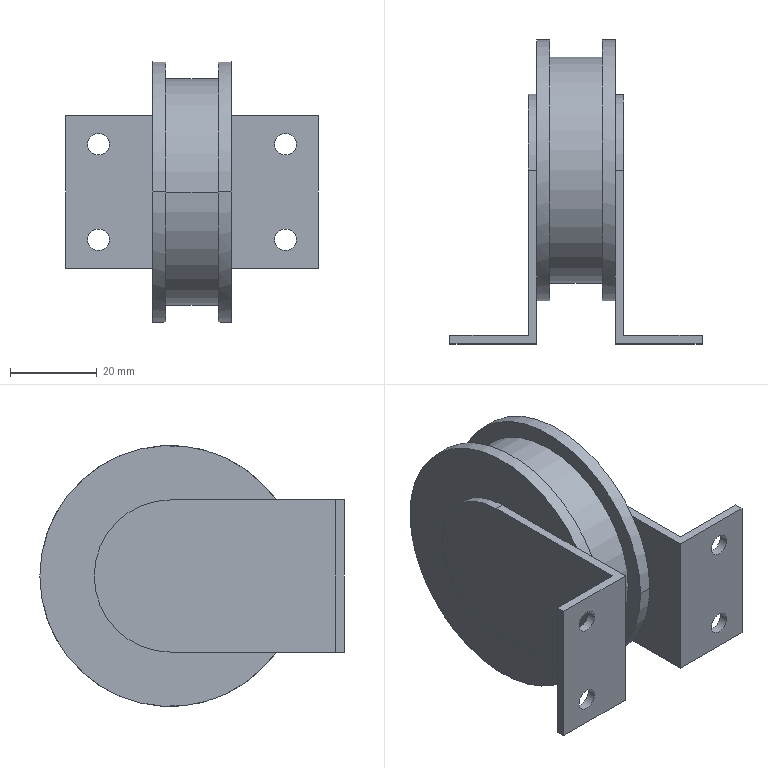Part | SolidWorks | features ICE 3, MirrorPattern 1, Revolution 1 | 1 solid | 35 faces | box 58 x 70 x 60 mm | volume 52336 mm3 | plane 18 | cylinder 17 | commonest cylinder face diameters 5 x8 60 x4 35 x3 52 x2
STEP:
#1=CARTESIAN_POINT('',(33.,-38.,11.));
#2=VERTEX_POINT('',#1);
#3=CARTESIAN_POINT('',(28.,-38.,11.));
#4=VERTEX_POINT('',#3);
#5=CARTESIAN_POINT('',(30.5,-38.,11.));
#6=DIRECTION('',(0.,1.,0.));
#7=DIRECTION('',(1.,0.,0.));
#8=AXIS2_PLACEMENT_3D('',#5,#6,#7);
#9=CIRCLE('',#8,2.5);
#10=EDGE_CURVE('',#2,#4,#9,.T.);
#11=ORIENTED_EDGE('',*,*,#10,.T.);
#12=CARTESIAN_POINT('',(28.,-40.,11.));
#13=VERTEX_POINT('',#12);
#14=CARTESIAN_POINT('',(28.,30.001,11.));
#15=DIRECTION('',(0.,-1.,0.));
#16=VECTOR('',#15,1000.);
#17=LINE('',#14,#16);
#18=EDGE_CURVE('',#4,#13,#17,.T.);
#19=ORIENTED_EDGE('',*,*,#18,.T.);
#20=CARTESIAN_POINT('',(33.,-40.,11.));
#21=VERTEX_POINT('',#20);
#22=CARTESIAN_POINT('',(30.5,-40.,11.));
#23=DIRECTION('',(0.,-1.,0.));
#24=DIRECTION('',(-1.,0.,0.));
#25=AXIS2_PLACEMENT_3D('',#22,#23,#24);
#26=CIRCLE('',#25,2.5);
#27=EDGE_CURVE('',#13,#21,#26,.T.);
#28=ORIENTED_EDGE('',*,*,#27,.T.);
#29=CARTESIAN_POINT('',(33.,30.001,11.));
#30=DIRECTION('',(0.,-1.,0.));
#31=VECTOR('',#30,1000.);
#32=LINE('',#29,#31);
#33=EDGE_CURVE('',#2,#21,#32,.T.);
#34=ORIENTED_EDGE('',*,*,#33,.F.);
#35=EDGE_LOOP('',(#11,#19,#28,#34));
#36=FACE_OUTER_BOUND('',#35,.T.);
#37=CARTESIAN_POINT('',(30.5,30.001,11.));
#38=DIRECTION('',(0.,-1.,0.));
#39=DIRECTION('',(1.,0.,0.));
#40=AXIS2_PLACEMENT_3D('',#37,#38,#39);
#41=CYLINDRICAL_SURFACE('',#40,2.5);
#42=ADVANCED_FACE('',(#36),#41,.F.);
#43=CARTESIAN_POINT('',(33.,-38.,-11.));
#44=VERTEX_POINT('',#43);
#45=CARTESIAN_POINT('',(28.,-38.,-11.));
#46=VERTEX_POINT('',#45);
#47=CARTESIAN_POINT('',(30.5,-38.,-11.));
#48=DIRECTION('',(0.,1.,0.));
#49=DIRECTION('',(1.,0.,0.));
#50=AXIS2_PLACEMENT_3D('',#47,#48,#49);
#51=CIRCLE('',#50,2.5);
#52=EDGE_CURVE('',#44,#46,#51,.T.);
#53=ORIENTED_EDGE('',*,*,#52,.T.);
#54=CARTESIAN_POINT('',(28.,-40.,-11.));
#55=VERTEX_POINT('',#54);
#56=CARTESIAN_POINT('',(28.,30.001,-11.));
#57=DIRECTION('',(0.,-1.,0.));
#58=VECTOR('',#57,1000.);
#59=LINE('',#56,#58);
#60=EDGE_CURVE('',#46,#55,#59,.T.);
#61=ORIENTED_EDGE('',*,*,#60,.T.);
#62=CARTESIAN_POINT('',(33.,-40.,-11.));
#63=VERTEX_POINT('',#62);
#64=CARTESIAN_POINT('',(30.5,-40.,-11.));
#65=DIRECTION('',(0.,-1.,0.));
#66=DIRECTION('',(1.,0.,0.));
#67=AXIS2_PLACEMENT_3D('',#64,#65,#66);
#68=CIRCLE('',#67,2.5);
#69=EDGE_CURVE('',#55,#63,#68,.T.);
#70=ORIENTED_EDGE('',*,*,#69,.T.);
#71=CARTESIAN_POINT('',(33.,30.001,-11.));
#72=DIRECTION('',(0.,-1.,0.));
#73=VECTOR('',#72,1000.);
#74=LINE('',#71,#73);
#75=EDGE_CURVE('',#44,#63,#74,.T.);
#76=ORIENTED_EDGE('',*,*,#75,.F.);
#77=EDGE_LOOP('',(#53,#61,#70,#76));
#78=FACE_OUTER_BOUND('',#77,.T.);
#79=CARTESIAN_POINT('',(30.5,30.001,-11.));
#80=DIRECTION('',(0.,-1.,0.));
#81=DIRECTION('',(1.,0.,0.));
#82=AXIS2_PLACEMENT_3D('',#79,#80,#81);
#83=CYLINDRICAL_SURFACE('',#82,2.5);
#84=ADVANCED_FACE('',(#78),#83,.F.);
#85=CARTESIAN_POINT('',(-15.,-38.,-11.));
#86=VERTEX_POINT('',#85);
#87=CARTESIAN_POINT('',(-10.,-38.,-11.));
#88=VERTEX_POINT('',#87);
#89=CARTESIAN_POINT('',(-12.5,-38.,-11.));
#90=DIRECTION('',(0.,-1.,0.));
#91=DIRECTION('',(-1.,0.,0.));
#92=AXIS2_PLACEMENT_3D('',#89,#90,#91);
#93=CIRCLE('',#92,2.5);
#94=EDGE_CURVE('',#86,#88,#93,.T.);
#95=ORIENTED_EDGE('',*,*,#94,.F.);
#96=CARTESIAN_POINT('',(-15.,-40.,-11.));
#97=VERTEX_POINT('',#96);
#98=CARTESIAN_POINT('',(-15.,30.001,-11.));
#99=DIRECTION('',(0.,-1.,0.));
#100=VECTOR('',#99,1000.);
#101=LINE('',#98,#100);
#102=EDGE_CURVE('',#86,#97,#101,.T.);
#103=ORIENTED_EDGE('',*,*,#102,.T.);
#104=CARTESIAN_POINT('',(-10.,-40.,-11.));
#105=VERTEX_POINT('',#104);
#106=CARTESIAN_POINT('',(-12.5,-40.,-11.));
#107=DIRECTION('',(0.,-1.,0.));
#108=DIRECTION('',(-1.,0.,0.));
#109=AXIS2_PLACEMENT_3D('',#106,#107,#108);
#110=CIRCLE('',#109,2.5);
#111=EDGE_CURVE('',#97,#105,#110,.T.);
#112=ORIENTED_EDGE('',*,*,#111,.T.);
#113=CARTESIAN_POINT('',(-10.,30.001,-11.));
#114=DIRECTION('',(0.,-1.,0.));
#115=VECTOR('',#114,1000.);
#116=LINE('',#113,#115);
#117=EDGE_CURVE('',#88,#105,#116,.T.);
#118=ORIENTED_EDGE('',*,*,#117,.F.);
#119=EDGE_LOOP('',(#95,#103,#112,#118));
#120=FACE_OUTER_BOUND('',#119,.T.);
#121=CARTESIAN_POINT('',(-12.5,30.001,-11.));
#122=DIRECTION('',(0.,-1.,0.));
#123=DIRECTION('',(1.,0.,0.));
#124=AXIS2_PLACEMENT_3D('',#121,#122,#123);
#125=CYLINDRICAL_SURFACE('',#124,2.5);
#126=ADVANCED_FACE('',(#120),#125,.F.);
#127=CARTESIAN_POINT('',(-15.,-38.,11.));
#128=VERTEX_POINT('',#127);
#129=CARTESIAN_POINT('',(-10.,-38.,11.));
#130=VERTEX_POINT('',#129);
#131=CARTESIAN_POINT('',(-12.5,-38.,11.));
#132=DIRECTION('',(0.,-1.,0.));
#133=DIRECTION('',(-1.,0.,0.));
#134=AXIS2_PLACEMENT_3D('',#131,#132,#133);
#135=CIRCLE('',#134,2.5);
#136=EDGE_CURVE('',#128,#130,#135,.T.);
#137=ORIENTED_EDGE('',*,*,#136,.F.);
#138=CARTESIAN_POINT('',(-15.,-40.,11.));
#139=VERTEX_POINT('',#138);
#140=CARTESIAN_POINT('',(-15.,30.001,11.));
#141=DIRECTION('',(0.,-1.,0.));
#142=VECTOR('',#141,1000.);
#143=LINE('',#140,#142);
#144=EDGE_CURVE('',#128,#139,#143,.T.);
#145=ORIENTED_EDGE('',*,*,#144,.T.);
#146=CARTESIAN_POINT('',(-10.,-40.,11.));
#147=VERTEX_POINT('',#146);
#148=CARTESIAN_POINT('',(-12.5,-40.,11.));
#149=DIRECTION('',(0.,-1.,0.));
#150=DIRECTION('',(1.,0.,0.));
#151=AXIS2_PLACEMENT_3D('',#148,#149,#150);
#152=CIRCLE('',#151,2.5);
#153=EDGE_CURVE('',#139,#147,#152,.T.);
#154=ORIENTED_EDGE('',*,*,#153,.T.);
#155=CARTESIAN_POINT('',(-10.,30.001,11.));
#156=DIRECTION('',(0.,-1.,0.));
#157=VECTOR('',#156,1000.);
#158=LINE('',#155,#157);
#159=EDGE_CURVE('',#130,#147,#158,.T.);
#160=ORIENTED_EDGE('',*,*,#159,.F.);
#161=EDGE_LOOP('',(#137,#145,#154,#160));
#162=FACE_OUTER_BOUND('',#161,.T.);
#163=CARTESIAN_POINT('',(-12.5,30.001,11.));
#164=DIRECTION('',(0.,-1.,0.));
#165=DIRECTION('',(1.,0.,0.));
#166=AXIS2_PLACEMENT_3D('',#163,#164,#165);
#167=CYLINDRICAL_SURFACE('',#166,2.5);
#168=ADVANCED_FACE('',(#162),#167,.F.);
#169=CARTESIAN_POINT('',(-2.,0.,-17.5));
#170=VERTEX_POINT('',#169);
#171=CARTESIAN_POINT('',(-2.,17.5,0.));
#172=VERTEX_POINT('',#171);
#173=CARTESIAN_POINT('',(-2.,0.,0.));
#174=DIRECTION('',(1.,0.,0.));
#175=DIRECTION('',(0.,1.,0.));
#176=AXIS2_PLACEMENT_3D('',#173,#174,#175);
#177=CIRCLE('',#176,17.5);
#178=EDGE_CURVE('',#170,#172,#177,.T.);
#179=ORIENTED_EDGE('',*,*,#178,.T.);
#180=CARTESIAN_POINT('',(0.,17.5,0.));
#181=VERTEX_POINT('',#180);
#182=CARTESIAN_POINT('',(-2.,17.5,0.));
#183=DIRECTION('',(1.,0.,0.));
#184=VECTOR('',#183,1000.);
#185=LINE('',#182,#184);
#186=EDGE_CURVE('',#172,#181,#185,.T.);
#187=ORIENTED_EDGE('',*,*,#186,.T.);
#188=CARTESIAN_POINT('',(0.,0.,-17.5));
#189=VERTEX_POINT('',#188);
#190=CARTESIAN_POINT('',(0.,0.,0.));
#191=DIRECTION('',(1.,0.,0.));
#192=DIRECTION('',(0.,1.,0.));
#193=AXIS2_PLACEMENT_3D('',#190,#191,#192);
#194=CIRCLE('',#193,17.5);
#195=EDGE_CURVE('',#189,#181,#194,.T.);
#196=ORIENTED_EDGE('',*,*,#195,.F.);
#197=CARTESIAN_POINT('',(-2.,0.,-17.5));
#198=DIRECTION('',(1.,0.,0.));
#199=VECTOR('',#198,1000.);
#200=LINE('',#197,#199);
#201=EDGE_CURVE('',#170,#189,#200,.T.);
#202=ORIENTED_EDGE('',*,*,#201,.F.);
#203=EDGE_LOOP('',(#179,#187,#196,#202));
#204=FACE_OUTER_BOUND('',#203,.T.);
#205=CARTESIAN_POINT('',(-2.,0.,0.));
#206=DIRECTION('',(1.,0.,0.));
#207=DIRECTION('',(0.,1.,0.));
#208=AXIS2_PLACEMENT_3D('',#205,#206,#207);
#209=CYLINDRICAL_SURFACE('',#208,17.5);
#210=ADVANCED_FACE('',(#204),#209,.T.);
#211=CARTESIAN_POINT('',(3.,26.,0.));
#212=VERTEX_POINT('',#211);
#213=CARTESIAN_POINT('',(3.,-26.,0.));
#214=VERTEX_POINT('',#213);
#215=CARTESIAN_POINT('',(3.,0.,0.));
#216=DIRECTION('',(1.,0.,0.));
#217=DIRECTION('',(0.,1.,0.));
#218=AXIS2_PLACEMENT_3D('',#215,#216,#217);
#219=CIRCLE('',#218,26.);
#220=EDGE_CURVE('',#212,#214,#219,.T.);
#221=ORIENTED_EDGE('',*,*,#220,.T.);
#222=CARTESIAN_POINT('',(15.,-26.,0.));
#223=VERTEX_POINT('',#222);
#224=CARTESIAN_POINT('',(18.,-26.,0.));
#225=DIRECTION('',(1.,0.,0.));
#226=VECTOR('',#225,1000.);
#227=LINE('',#224,#226);
#228=EDGE_CURVE('',#214,#223,#227,.T.);
#229=ORIENTED_EDGE('',*,*,#228,.T.);
#230=CARTESIAN_POINT('',(15.,26.,0.));
#231=VERTEX_POINT('',#230);
#232=CARTESIAN_POINT('',(15.,0.,0.));
#233=DIRECTION('',(1.,0.,0.));
#234=DIRECTION('',(0.,1.,0.));
#235=AXIS2_PLACEMENT_3D('',#232,#233,#234);
#236=CIRCLE('',#235,26.);
#237=EDGE_CURVE('',#231,#223,#236,.T.);
#238=ORIENTED_EDGE('',*,*,#237,.F.);
#239=CARTESIAN_POINT('',(18.,26.,0.));
#240=DIRECTION('',(1.,0.,0.));
#241=VECTOR('',#240,1000.);
#242=LINE('',#239,#241);
#243=EDGE_CURVE('',#212,#231,#242,.T.);
#244=ORIENTED_EDGE('',*,*,#243,.F.);
#245=EDGE_LOOP('',(#221,#229,#238,#244));
#246=FACE_OUTER_BOUND('',#245,.T.);
#247=CARTESIAN_POINT('',(18.,0.,0.));
#248=DIRECTION('',(1.,0.,0.));
#249=DIRECTION('',(0.,1.,0.));
#250=AXIS2_PLACEMENT_3D('',#247,#248,#249);
#251=CYLINDRICAL_SURFACE('',#250,26.);
#252=ADVANCED_FACE('',(#246),#251,.T.);
#253=CARTESIAN_POINT('',(15.,30.,0.));
#254=VERTEX_POINT('',#253);
#255=CARTESIAN_POINT('',(15.,-30.,0.));
#256=VERTEX_POINT('',#255);
#257=CARTESIAN_POINT('',(15.,0.,0.));
#258=DIRECTION('',(1.,0.,0.));
#259=DIRECTION('',(0.,1.,0.));
#260=AXIS2_PLACEMENT_3D('',#257,#258,#259);
#261=CIRCLE('',#260,30.);
#262=EDGE_CURVE('',#254,#256,#261,.T.);
#263=ORIENTED_EDGE('',*,*,#262,.T.);
#264=CARTESIAN_POINT('',(18.,-30.,0.));
#265=VERTEX_POINT('',#264);
#266=CARTESIAN_POINT('',(18.,-30.,0.));
#267=DIRECTION('',(1.,0.,0.));
#268=VECTOR('',#267,1000.);
#269=LINE('',#266,#268);
#270=EDGE_CURVE('',#256,#265,#269,.T.);
#271=ORIENTED_EDGE('',*,*,#270,.T.);
#272=CARTESIAN_POINT('',(18.,-24.367,17.5));
#273=VERTEX_POINT('',#272);
#274=CARTESIAN_POINT('',(18.,0.,0.));
#275=DIRECTION('',(1.,0.,0.));
#276=DIRECTION('',(0.,1.,0.));
#277=AXIS2_PLACEMENT_3D('',#274,#275,#276);
#278=CIRCLE('',#277,30.);
#279=EDGE_CURVE('',#273,#265,#278,.T.);
#280=ORIENTED_EDGE('',*,*,#279,.F.);
#281=CARTESIAN_POINT('',(18.,30.,0.));
#282=VERTEX_POINT('',#281);
#283=CARTESIAN_POINT('',(18.,0.,0.));
#284=DIRECTION('',(1.,0.,0.));
#285=DIRECTION('',(0.,1.,0.));
#286=AXIS2_PLACEMENT_3D('',#283,#284,#285);
#287=CIRCLE('',#286,30.);
#288=EDGE_CURVE('',#282,#273,#287,.T.);
#289=ORIENTED_EDGE('',*,*,#288,.F.);
#290=CARTESIAN_POINT('',(18.,30.,0.));
#291=DIRECTION('',(1.,0.,0.));
#292=VECTOR('',#291,1000.);
#293=LINE('',#290,#292);
#294=EDGE_CURVE('',#254,#282,#293,.T.);
#295=ORIENTED_EDGE('',*,*,#294,.F.);
#296=EDGE_LOOP('',(#263,#271,#280,#289,#295));
#297=FACE_OUTER_BOUND('',#296,.T.);
#298=CARTESIAN_POINT('',(18.,0.,0.));
#299=DIRECTION('',(1.,0.,0.));
#300=DIRECTION('',(0.,1.,0.));
#301=AXIS2_PLACEMENT_3D('',#298,#299,#300);
#302=CYLINDRICAL_SURFACE('',#301,30.);
#303=ADVANCED_FACE('',(#297),#302,.T.);
#304=CARTESIAN_POINT('',(0.,-24.367,17.5));
#305=VERTEX_POINT('',#304);
#306=CARTESIAN_POINT('',(0.,-30.,0.));
#307=VERTEX_POINT('',#306);
#308=CARTESIAN_POINT('',(0.,0.,0.));
#309=DIRECTION('',(1.,0.,0.));
#310=DIRECTION('',(0.,1.,0.));
#311=AXIS2_PLACEMENT_3D('',#308,#309,#310);
#312=CIRCLE('',#311,30.);
#313=EDGE_CURVE('',#305,#307,#312,.T.);
#314=ORIENTED_EDGE('',*,*,#313,.T.);
#315=CARTESIAN_POINT('',(3.,-30.,0.));
#316=VERTEX_POINT('',#315);
#317=CARTESIAN_POINT('',(18.,-30.,0.));
#318=DIRECTION('',(1.,0.,0.));
#319=VECTOR('',#318,1000.);
#320=LINE('',#317,#319);
#321=EDGE_CURVE('',#307,#316,#320,.T.);
#322=ORIENTED_EDGE('',*,*,#321,.T.);
#323=CARTESIAN_POINT('',(3.,30.,0.));
#324=VERTEX_POINT('',#323);
#325=CARTESIAN_POINT('',(3.,0.,0.));
#326=DIRECTION('',(1.,0.,0.));
#327=DIRECTION('',(0.,1.,0.));
#328=AXIS2_PLACEMENT_3D('',#325,#326,#327);
#329=CIRCLE('',#328,30.);
#330=EDGE_CURVE('',#324,#316,#329,.T.);
#331=ORIENTED_EDGE('',*,*,#330,.F.);
#332=CARTESIAN_POINT('',(0.,30.,0.));
#333=VERTEX_POINT('',#332);
#334=CARTESIAN_POINT('',(18.,30.,0.));
#335=DIRECTION('',(1.,0.,0.));
#336=VECTOR('',#335,1000.);
#337=LINE('',#334,#336);
#338=EDGE_CURVE('',#333,#324,#337,.T.);
#339=ORIENTED_EDGE('',*,*,#338,.F.);
#340=CARTESIAN_POINT('',(0.,0.,0.));
#341=DIRECTION('',(1.,0.,0.));
#342=DIRECTION('',(0.,1.,0.));
#343=AXIS2_PLACEMENT_3D('',#340,#341,#342);
#344=CIRCLE('',#343,30.);
#345=EDGE_CURVE('',#333,#305,#344,.T.);
#346=ORIENTED_EDGE('',*,*,#345,.T.);
#347=EDGE_LOOP('',(#314,#322,#331,#339,#346));
#348=FACE_OUTER_BOUND('',#347,.T.);
#349=CARTESIAN_POINT('',(18.,0.,0.));
#350=DIRECTION('',(1.,0.,0.));
#351=DIRECTION('',(0.,1.,0.));
#352=AXIS2_PLACEMENT_3D('',#349,#350,#351);
#353=CYLINDRICAL_SURFACE('',#352,30.);
#354=ADVANCED_FACE('',(#348),#353,.T.);
#355=CARTESIAN_POINT('',(-2.,-38.,-17.5));
#356=VERTEX_POINT('',#355);
#357=CARTESIAN_POINT('',(-2.,0.,-17.5));
#358=DIRECTION('',(0.,1.,0.));
#359=VECTOR('',#358,1000.);
#360=LINE('',#357,#359);
#361=EDGE_CURVE('',#356,#170,#360,.T.);
#362=ORIENTED_EDGE('',*,*,#361,.F.);
#363=CARTESIAN_POINT('',(-2.,-38.,17.5));
#364=VERTEX_POINT('',#363);
#365=CARTESIAN_POINT('',(-2.,-38.,17.5));
#366=DIRECTION('',(0.,0.,1.));
#367=VECTOR('',#366,1000.);
#368=LINE('',#365,#367);
#369=EDGE_CURVE('',#356,#364,#368,.T.);
#370=ORIENTED_EDGE('',*,*,#369,.T.);
#371=CARTESIAN_POINT('',(-2.,0.,17.5));
#372=VERTEX_POINT('',#371);
#373=CARTESIAN_POINT('',(-2.,0.,17.5));
#374=DIRECTION('',(0.,-1.,0.));
#375=VECTOR('',#374,1000.);
#376=LINE('',#373,#375);
#377=EDGE_CURVE('',#372,#364,#376,.T.);
#378=ORIENTED_EDGE('',*,*,#377,.F.);
#379=CARTESIAN_POINT('',(-2.,0.,0.));
#380=DIRECTION('',(1.,0.,0.));
#381=DIRECTION('',(0.,1.,0.));
#382=AXIS2_PLACEMENT_3D('',#379,#380,#381);
#383=CIRCLE('',#382,17.5);
#384=EDGE_CURVE('',#172,#372,#383,.T.);
#385=ORIENTED_EDGE('',*,*,#384,.F.);
#386=ORIENTED_EDGE('',*,*,#178,.F.);
#387=EDGE_LOOP('',(#362,#370,#378,#385,#386));
#388=FACE_OUTER_BOUND('',#387,.T.);
#389=CARTESIAN_POINT('',(-2.,0.,0.));
#390=DIRECTION('',(-1.,0.,0.));
#391=DIRECTION('',(0.,1.,0.));
#392=AXIS2_PLACEMENT_3D('',#389,#390,#391);
#393=PLANE('',#392);
#394=ADVANCED_FACE('',(#388),#393,.T.);
#395=ORIENTED_EDGE('',*,*,#195,.T.);
#396=CARTESIAN_POINT('',(0.,0.,17.5));
#397=VERTEX_POINT('',#396);
#398=CARTESIAN_POINT('',(0.,0.,0.));
#399=DIRECTION('',(1.,0.,0.));
#400=DIRECTION('',(0.,1.,0.));
#401=AXIS2_PLACEMENT_3D('',#398,#399,#400);
#402=CIRCLE('',#401,17.5);
#403=EDGE_CURVE('',#181,#397,#402,.T.);
#404=ORIENTED_EDGE('',*,*,#403,.T.);
#405=CARTESIAN_POINT('',(0.,0.,17.5));
#406=DIRECTION('',(0.,-1.,0.));
#407=VECTOR('',#406,1000.);
#408=LINE('',#405,#407);
#409=EDGE_CURVE('',#397,#305,#408,.T.);
#410=ORIENTED_EDGE('',*,*,#409,.T.);
#411=ORIENTED_EDGE('',*,*,#345,.F.);
#412=CARTESIAN_POINT('',(0.,-24.367,-17.5));
#413=VERTEX_POINT('',#412);
#414=CARTESIAN_POINT('',(0.,0.,0.));
#415=DIRECTION('',(1.,0.,0.));
#416=DIRECTION('',(0.,1.,0.));
#417=AXIS2_PLACEMENT_3D('',#414,#415,#416);
#418=CIRCLE('',#417,30.);
#419=EDGE_CURVE('',#413,#333,#418,.T.);
#420=ORIENTED_EDGE('',*,*,#419,.F.);
#421=CARTESIAN_POINT('',(0.,0.,-17.5));
#422=DIRECTION('',(0.,1.,0.));
#423=VECTOR('',#422,1000.);
#424=LINE('',#421,#423);
#425=EDGE_CURVE('',#413,#189,#424,.T.);
#426=ORIENTED_EDGE('',*,*,#425,.T.);
#427=EDGE_LOOP('',(#395,#404,#410,#411,#420,#426));
#428=FACE_OUTER_BOUND('',#427,.T.);
#429=CARTESIAN_POINT('',(0.,0.,0.));
#430=DIRECTION('',(-1.,0.,0.));
#431=DIRECTION('',(0.,-1.,0.));
#432=AXIS2_PLACEMENT_3D('',#429,#430,#431);
#433=PLANE('',#432);
#434=ADVANCED_FACE('',(#428),#433,.T.);
#435=CARTESIAN_POINT('',(18.,-24.367,-17.5));
#436=VERTEX_POINT('',#435);
#437=CARTESIAN_POINT('',(18.,0.,-17.5));
#438=VERTEX_POINT('',#437);
#439=CARTESIAN_POINT('',(18.,0.,-17.5));
#440=DIRECTION('',(0.,1.,0.));
#441=VECTOR('',#440,1000.);
#442=LINE('',#439,#441);
#443=EDGE_CURVE('',#436,#438,#442,.T.);
#444=ORIENTED_EDGE('',*,*,#443,.F.);
#445=CARTESIAN_POINT('',(18.,0.,0.));
#446=DIRECTION('',(1.,0.,0.));
#447=DIRECTION('',(0.,1.,0.));
#448=AXIS2_PLACEMENT_3D('',#445,#446,#447);
#449=CIRCLE('',#448,30.);
#450=EDGE_CURVE('',#436,#282,#449,.T.);
#451=ORIENTED_EDGE('',*,*,#450,.T.);
#452=ORIENTED_EDGE('',*,*,#288,.T.);
#453=CARTESIAN_POINT('',(18.,0.,17.5));
#454=VERTEX_POINT('',#453);
#455=CARTESIAN_POINT('',(18.,0.,17.5));
#456=DIRECTION('',(0.,-1.,0.));
#457=VECTOR('',#456,1000.);
#458=LINE('',#455,#457);
#459=EDGE_CURVE('',#454,#273,#458,.T.);
#460=ORIENTED_EDGE('',*,*,#459,.F.);
#461=CARTESIAN_POINT('',(18.,0.,0.));
#462=DIRECTION('',(1.,0.,0.));
#463=DIRECTION('',(0.,1.,0.));
#464=AXIS2_PLACEMENT_3D('',#461,#462,#463);
#465=CIRCLE('',#464,17.5);
#466=EDGE_CURVE('',#438,#454,#465,.T.);
#467=ORIENTED_EDGE('',*,*,#466,.F.);
#468=EDGE_LOOP('',(#444,#451,#452,#460,#467));
#469=FACE_OUTER_BOUND('',#468,.T.);
#470=CARTESIAN_POINT('',(18.,0.,0.));
#471=DIRECTION('',(-1.,0.,0.));
#472=DIRECTION('',(0.,-1.,0.));
#473=AXIS2_PLACEMENT_3D('',#470,#471,#472);
#474=PLANE('',#473);
#475=ADVANCED_FACE('',(#469),#474,.F.);
#476=ORIENTED_EDGE('',*,*,#321,.F.);
#477=CARTESIAN_POINT('',(0.,0.,0.));
#478=DIRECTION('',(1.,0.,0.));
#479=DIRECTION('',(0.,1.,0.));
#480=AXIS2_PLACEMENT_3D('',#477,#478,#479);
#481=CIRCLE('',#480,30.);
#482=EDGE_CURVE('',#307,#413,#481,.T.);
#483=ORIENTED_EDGE('',*,*,#482,.T.);
#484=ORIENTED_EDGE('',*,*,#419,.T.);
#485=ORIENTED_EDGE('',*,*,#338,.T.);
#486=CARTESIAN_POINT('',(3.,0.,0.));
#487=DIRECTION('',(1.,0.,0.));
#488=DIRECTION('',(0.,1.,0.));
#489=AXIS2_PLACEMENT_3D('',#486,#487,#488);
#490=CIRCLE('',#489,30.);
#491=EDGE_CURVE('',#316,#324,#490,.T.);
#492=ORIENTED_EDGE('',*,*,#491,.F.);
#493=EDGE_LOOP('',(#476,#483,#484,#485,#492));
#494=FACE_OUTER_BOUND('',#493,.T.);
#495=CARTESIAN_POINT('',(18.,0.,0.));
#496=DIRECTION('',(1.,0.,0.));
#497=DIRECTION('',(0.,1.,0.));
#498=AXIS2_PLACEMENT_3D('',#495,#496,#497);
#499=CYLINDRICAL_SURFACE('',#498,30.);
#500=ADVANCED_FACE('',(#494),#499,.T.);
#501=ORIENTED_EDGE('',*,*,#270,.F.);
#502=CARTESIAN_POINT('',(15.,0.,0.));
#503=DIRECTION('',(1.,0.,0.));
#504=DIRECTION('',(0.,1.,0.));
#505=AXIS2_PLACEMENT_3D('',#502,#503,#504);
#506=CIRCLE('',#505,30.);
#507=EDGE_CURVE('',#256,#254,#506,.T.);
#508=ORIENTED_EDGE('',*,*,#507,.T.);
#509=ORIENTED_EDGE('',*,*,#294,.T.);
#510=ORIENTED_EDGE('',*,*,#450,.F.);
#511=CARTESIAN_POINT('',(18.,0.,0.));
#512=DIRECTION('',(1.,0.,0.));
#513=DIRECTION('',(0.,1.,0.));
#514=AXIS2_PLACEMENT_3D('',#511,#512,#513);
#515=CIRCLE('',#514,30.);
#516=EDGE_CURVE('',#265,#436,#515,.T.);
#517=ORIENTED_EDGE('',*,*,#516,.F.);
#518=EDGE_LOOP('',(#501,#508,#509,#510,#517));
#519=FACE_OUTER_BOUND('',#518,.T.);
#520=CARTESIAN_POINT('',(18.,0.,0.));
#521=DIRECTION('',(1.,0.,0.));
#522=DIRECTION('',(0.,1.,0.));
#523=AXIS2_PLACEMENT_3D('',#520,#521,#522);
#524=CYLINDRICAL_SURFACE('',#523,30.);
#525=ADVANCED_FACE('',(#519),#524,.T.);
#526=ORIENTED_EDGE('',*,*,#262,.F.);
#527=ORIENTED_EDGE('',*,*,#507,.F.);
#528=EDGE_LOOP('',(#526,#527));
#529=FACE_OUTER_BOUND('',#528,.T.);
#530=ORIENTED_EDGE('',*,*,#237,.T.);
#531=CARTESIAN_POINT('',(15.,0.,0.));
#532=DIRECTION('',(1.,0.,0.));
#533=DIRECTION('',(0.,1.,0.));
#534=AXIS2_PLACEMENT_3D('',#531,#532,#533);
#535=CIRCLE('',#534,26.);
#536=EDGE_CURVE('',#223,#231,#535,.T.);
#537=ORIENTED_EDGE('',*,*,#536,.T.);
#538=EDGE_LOOP('',(#530,#537));
#539=FACE_BOUND('',#538,.T.);
#540=CARTESIAN_POINT('',(15.,0.,0.));
#541=DIRECTION('',(1.,0.,0.));
#542=DIRECTION('',(0.,1.,0.));
#543=AXIS2_PLACEMENT_3D('',#540,#541,#542);
#544=PLANE('',#543);
#545=ADVANCED_FACE('',(#529,#539),#544,.F.);
#546=ORIENTED_EDGE('',*,*,#228,.F.);
#547=CARTESIAN_POINT('',(3.,0.,0.));
#548=DIRECTION('',(1.,0.,0.));
#549=DIRECTION('',(0.,1.,0.));
#550=AXIS2_PLACEMENT_3D('',#547,#548,#549);
#551=CIRCLE('',#550,26.);
#552=EDGE_CURVE('',#214,#212,#551,.T.);
#553=ORIENTED_EDGE('',*,*,#552,.T.);
#554=ORIENTED_EDGE('',*,*,#243,.T.);
#555=ORIENTED_EDGE('',*,*,#536,.F.);
#556=EDGE_LOOP('',(#546,#553,#554,#555));
#557=FACE_OUTER_BOUND('',#556,.T.);
#558=CARTESIAN_POINT('',(18.,0.,0.));
#559=DIRECTION('',(1.,0.,0.));
#560=DIRECTION('',(0.,1.,0.));
#561=AXIS2_PLACEMENT_3D('',#558,#559,#560);
#562=CYLINDRICAL_SURFACE('',#561,26.);
#563=ADVANCED_FACE('',(#557),#562,.T.);
#564=ORIENTED_EDGE('',*,*,#220,.F.);
#565=ORIENTED_EDGE('',*,*,#552,.F.);
#566=EDGE_LOOP('',(#564,#565));
#567=FACE_BOUND('',#566,.T.);
#568=ORIENTED_EDGE('',*,*,#330,.T.);
#569=ORIENTED_EDGE('',*,*,#491,.T.);
#570=EDGE_LOOP('',(#568,#569));
#571=FACE_OUTER_BOUND('',#570,.T.);
#572=CARTESIAN_POINT('',(3.,0.,0.));
#573=DIRECTION('',(-1.,0.,0.));
#574=DIRECTION('',(0.,-1.,0.));
#575=AXIS2_PLACEMENT_3D('',#572,#573,#574);
#576=PLANE('',#575);
#577=ADVANCED_FACE('',(#567,#571),#576,.F.);
#578=CARTESIAN_POINT('',(18.,-40.,17.5));
#579=VERTEX_POINT('',#578);
#580=CARTESIAN_POINT('',(18.,0.,17.5));
#581=DIRECTION('',(0.,-1.,0.));
#582=VECTOR('',#581,1000.);
#583=LINE('',#580,#582);
#584=EDGE_CURVE('',#273,#579,#583,.T.);
#585=ORIENTED_EDGE('',*,*,#584,.F.);
#586=ORIENTED_EDGE('',*,*,#279,.T.);
#587=ORIENTED_EDGE('',*,*,#516,.T.);
#588=CARTESIAN_POINT('',(18.,-40.,-17.5));
#589=VERTEX_POINT('',#588);
#590=CARTESIAN_POINT('',(18.,0.,-17.5));
#591=DIRECTION('',(0.,1.,0.));
#592=VECTOR('',#591,1000.);
#593=LINE('',#590,#592);
#594=EDGE_CURVE('',#589,#436,#593,.T.);
#595=ORIENTED_EDGE('',*,*,#594,.F.);
#596=CARTESIAN_POINT('',(18.,-40.,0.));
#597=DIRECTION('',(0.,0.,-1.));
#598=VECTOR('',#597,1000.);
#599=LINE('',#596,#598);
#600=EDGE_CURVE('',#579,#589,#599,.T.);
#601=ORIENTED_EDGE('',*,*,#600,.F.);
#602=EDGE_LOOP('',(#585,#586,#587,#595,#601));
#603=FACE_OUTER_BOUND('',#602,.T.);
#604=CARTESIAN_POINT('',(18.,0.,0.));
#605=DIRECTION('',(1.,0.,0.));
#606=DIRECTION('',(0.,1.,0.));
#607=AXIS2_PLACEMENT_3D('',#604,#605,#606);
#608=PLANE('',#607);
#609=ADVANCED_FACE('',(#603),#608,.F.);
#610=ORIENTED_EDGE('',*,*,#466,.T.);
#611=CARTESIAN_POINT('',(20.,0.,17.5));
#612=VERTEX_POINT('',#611);
#613=CARTESIAN_POINT('',(20.,0.,17.5));
#614=DIRECTION('',(-1.,0.,0.));
#615=VECTOR('',#614,1000.);
#616=LINE('',#613,#615);
#617=EDGE_CURVE('',#612,#454,#616,.T.);
#618=ORIENTED_EDGE('',*,*,#617,.F.);
#619=CARTESIAN_POINT('',(20.,0.,-17.5));
#620=VERTEX_POINT('',#619);
#621=CARTESIAN_POINT('',(20.,0.,0.));
#622=DIRECTION('',(1.,0.,0.));
#623=DIRECTION('',(0.,1.,0.));
#624=AXIS2_PLACEMENT_3D('',#621,#622,#623);
#625=CIRCLE('',#624,17.5);
#626=EDGE_CURVE('',#620,#612,#625,.T.);
#627=ORIENTED_EDGE('',*,*,#626,.F.);
#628=CARTESIAN_POINT('',(20.,0.,-17.5));
#629=DIRECTION('',(-1.,0.,0.));
#630=VECTOR('',#629,1000.);
#631=LINE('',#628,#630);
#632=EDGE_CURVE('',#620,#438,#631,.T.);
#633=ORIENTED_EDGE('',*,*,#632,.T.);
#634=EDGE_LOOP('',(#610,#618,#627,#633));
#635=FACE_OUTER_BOUND('',#634,.T.);
#636=CARTESIAN_POINT('',(20.,0.,0.));
#637=DIRECTION('',(-1.,0.,0.));
#638=DIRECTION('',(0.,-1.,0.));
#639=AXIS2_PLACEMENT_3D('',#636,#637,#638);
#640=CYLINDRICAL_SURFACE('',#639,17.5);
#641=ADVANCED_FACE('',(#635),#640,.T.);
#642=ORIENTED_EDGE('',*,*,#459,.T.);
#643=ORIENTED_EDGE('',*,*,#584,.T.);
#644=CARTESIAN_POINT('',(38.,-40.,17.5));
#645=VERTEX_POINT('',#644);
#646=CARTESIAN_POINT('',(20.,-40.,17.5));
#647=DIRECTION('',(-1.,0.,0.));
#648=VECTOR('',#647,1000.);
#649=LINE('',#646,#648);
#650=EDGE_CURVE('',#645,#579,#649,.T.);
#651=ORIENTED_EDGE('',*,*,#650,.F.);
#652=CARTESIAN_POINT('',(38.,-38.,17.5));
#653=VERTEX_POINT('',#652);
#654=CARTESIAN_POINT('',(38.,-40.,17.5));
#655=DIRECTION('',(0.,-1.,0.));
#656=VECTOR('',#655,1000.);
#657=LINE('',#654,#656);
#658=EDGE_CURVE('',#653,#645,#657,.T.);
#659=ORIENTED_EDGE('',*,*,#658,.F.);
#660=CARTESIAN_POINT('',(20.,-38.,17.5));
#661=VERTEX_POINT('',#660);
#662=CARTESIAN_POINT('',(38.,-38.,17.5));
#663=DIRECTION('',(-1.,0.,0.));
#664=VECTOR('',#663,1000.);
#665=LINE('',#662,#664);
#666=EDGE_CURVE('',#653,#661,#665,.T.);
#667=ORIENTED_EDGE('',*,*,#666,.T.);
#668=CARTESIAN_POINT('',(20.,0.,17.5));
#669=DIRECTION('',(0.,-1.,0.));
#670=VECTOR('',#669,1000.);
#671=LINE('',#668,#670);
#672=EDGE_CURVE('',#612,#661,#671,.T.);
#673=ORIENTED_EDGE('',*,*,#672,.F.);
#674=ORIENTED_EDGE('',*,*,#617,.T.);
#675=EDGE_LOOP('',(#642,#643,#651,#659,#667,#673,#674));
#676=FACE_OUTER_BOUND('',#675,.T.);
#677=CARTESIAN_POINT('',(20.,0.,17.5));
#678=DIRECTION('',(0.,0.,-1.));
#679=DIRECTION('',(0.,1.,0.));
#680=AXIS2_PLACEMENT_3D('',#677,#678,#679);
#681=PLANE('',#680);
#682=ADVANCED_FACE('',(#676),#681,.F.);
#683=CARTESIAN_POINT('',(30.5,-40.,11.));
#684=DIRECTION('',(0.,-1.,0.));
#685=DIRECTION('',(-1.,0.,0.));
#686=AXIS2_PLACEMENT_3D('',#683,#684,#685);
#687=CIRCLE('',#686,2.5);
#688=EDGE_CURVE('',#21,#13,#687,.T.);
#689=ORIENTED_EDGE('',*,*,#688,.F.);
#690=ORIENTED_EDGE('',*,*,#27,.F.);
#691=EDGE_LOOP('',(#689,#690));
#692=FACE_BOUND('',#691,.T.);
#693=CARTESIAN_POINT('',(30.5,-40.,-11.));
#694=DIRECTION('',(0.,-1.,0.));
#695=DIRECTION('',(1.,0.,0.));
#696=AXIS2_PLACEMENT_3D('',#693,#694,#695);
#697=CIRCLE('',#696,2.5);
#698=EDGE_CURVE('',#63,#55,#697,.T.);
#699=ORIENTED_EDGE('',*,*,#698,.F.);
#700=ORIENTED_EDGE('',*,*,#69,.F.);
#701=EDGE_LOOP('',(#699,#700));
#702=FACE_BOUND('',#701,.T.);
#703=ORIENTED_EDGE('',*,*,#600,.T.);
#704=CARTESIAN_POINT('',(38.,-40.,-17.5));
#705=VERTEX_POINT('',#704);
#706=CARTESIAN_POINT('',(20.,-40.,-17.5));
#707=DIRECTION('',(-1.,0.,0.));
#708=VECTOR('',#707,1000.);
#709=LINE('',#706,#708);
#710=EDGE_CURVE('',#705,#589,#709,.T.);
#711=ORIENTED_EDGE('',*,*,#710,.F.);
#712=CARTESIAN_POINT('',(38.,-40.,17.5));
#713=DIRECTION('',(0.,0.,-1.));
#714=VECTOR('',#713,1000.);
#715=LINE('',#712,#714);
#716=EDGE_CURVE('',#645,#705,#715,.T.);
#717=ORIENTED_EDGE('',*,*,#716,.F.);
#718=ORIENTED_EDGE('',*,*,#650,.T.);
#719=EDGE_LOOP('',(#703,#711,#717,#718));
#720=FACE_OUTER_BOUND('',#719,.T.);
#721=CARTESIAN_POINT('',(20.,-40.,0.));
#722=DIRECTION('',(0.,1.,0.));
#723=DIRECTION('',(-1.,0.,0.));
#724=AXIS2_PLACEMENT_3D('',#721,#722,#723);
#725=PLANE('',#724);
#726=ADVANCED_FACE('',(#692,#702,#720),#725,.F.);
#727=ORIENTED_EDGE('',*,*,#594,.T.);
#728=ORIENTED_EDGE('',*,*,#443,.T.);
#729=ORIENTED_EDGE('',*,*,#632,.F.);
#730=CARTESIAN_POINT('',(20.,-38.,-17.5));
#731=VERTEX_POINT('',#730);
#732=CARTESIAN_POINT('',(20.,0.,-17.5));
#733=DIRECTION('',(0.,1.,0.));
#734=VECTOR('',#733,1000.);
#735=LINE('',#732,#734);
#736=EDGE_CURVE('',#731,#620,#735,.T.);
#737=ORIENTED_EDGE('',*,*,#736,.F.);
#738=CARTESIAN_POINT('',(38.,-38.,-17.5));
#739=VERTEX_POINT('',#738);
#740=CARTESIAN_POINT('',(38.,-38.,-17.5));
#741=DIRECTION('',(-1.,0.,0.));
#742=VECTOR('',#741,1000.);
#743=LINE('',#740,#742);
#744=EDGE_CURVE('',#739,#731,#743,.T.);
#745=ORIENTED_EDGE('',*,*,#744,.F.);
#746=CARTESIAN_POINT('',(38.,-40.,-17.5));
#747=DIRECTION('',(0.,1.,0.));
#748=VECTOR('',#747,1000.);
#749=LINE('',#746,#748);
#750=EDGE_CURVE('',#705,#739,#749,.T.);
#751=ORIENTED_EDGE('',*,*,#750,.F.);
#752=ORIENTED_EDGE('',*,*,#710,.T.);
#753=EDGE_LOOP('',(#727,#728,#729,#737,#745,#751,#752));
#754=FACE_OUTER_BOUND('',#753,.T.);
#755=CARTESIAN_POINT('',(20.,0.,-17.5));
#756=DIRECTION('',(0.,0.,1.));
#757=DIRECTION('',(0.,-1.,0.));
#758=AXIS2_PLACEMENT_3D('',#755,#756,#757);
#759=PLANE('',#758);
#760=ADVANCED_FACE('',(#754),#759,.F.);
#761=CARTESIAN_POINT('',(20.,-38.,17.5));
#762=DIRECTION('',(0.,0.,1.));
#763=VECTOR('',#762,1000.);
#764=LINE('',#761,#763);
#765=EDGE_CURVE('',#731,#661,#764,.T.);
#766=ORIENTED_EDGE('',*,*,#765,.F.);
#767=ORIENTED_EDGE('',*,*,#736,.T.);
#768=ORIENTED_EDGE('',*,*,#626,.T.);
#769=ORIENTED_EDGE('',*,*,#672,.T.);
#770=EDGE_LOOP('',(#766,#767,#768,#769));
#771=FACE_OUTER_BOUND('',#770,.T.);
#772=CARTESIAN_POINT('',(20.,0.,0.));
#773=DIRECTION('',(1.,0.,0.));
#774=DIRECTION('',(0.,1.,0.));
#775=AXIS2_PLACEMENT_3D('',#772,#773,#774);
#776=PLANE('',#775);
#777=ADVANCED_FACE('',(#771),#776,.T.);
#778=ORIENTED_EDGE('',*,*,#10,.F.);
#779=CARTESIAN_POINT('',(30.5,-38.,11.));
#780=DIRECTION('',(0.,1.,0.));
#781=DIRECTION('',(1.,0.,0.));
#782=AXIS2_PLACEMENT_3D('',#779,#780,#781);
#783=CIRCLE('',#782,2.5);
#784=EDGE_CURVE('',#4,#2,#783,.T.);
#785=ORIENTED_EDGE('',*,*,#784,.F.);
#786=EDGE_LOOP('',(#778,#785));
#787=FACE_BOUND('',#786,.T.);
#788=ORIENTED_EDGE('',*,*,#52,.F.);
#789=CARTESIAN_POINT('',(30.5,-38.,-11.));
#790=DIRECTION('',(0.,1.,0.));
#791=DIRECTION('',(1.,0.,0.));
#792=AXIS2_PLACEMENT_3D('',#789,#790,#791);
#793=CIRCLE('',#792,2.5);
#794=EDGE_CURVE('',#46,#44,#793,.T.);
#795=ORIENTED_EDGE('',*,*,#794,.F.);
#796=EDGE_LOOP('',(#788,#795));
#797=FACE_BOUND('',#796,.T.);
#798=ORIENTED_EDGE('',*,*,#765,.T.);
#799=ORIENTED_EDGE('',*,*,#666,.F.);
#800=CARTESIAN_POINT('',(38.,-38.,17.5));
#801=DIRECTION('',(0.,0.,1.));
#802=VECTOR('',#801,1000.);
#803=LINE('',#800,#802);
#804=EDGE_CURVE('',#739,#653,#803,.T.);
#805=ORIENTED_EDGE('',*,*,#804,.F.);
#806=ORIENTED_EDGE('',*,*,#744,.T.);
#807=EDGE_LOOP('',(#798,#799,#805,#806));
#808=FACE_OUTER_BOUND('',#807,.T.);
#809=CARTESIAN_POINT('',(38.,-38.,17.5));
#810=DIRECTION('',(0.,-1.,0.));
#811=DIRECTION('',(1.,0.,0.));
#812=AXIS2_PLACEMENT_3D('',#809,#810,#811);
#813=PLANE('',#812);
#814=ADVANCED_FACE('',(#787,#797,#808),#813,.F.);
#815=ORIENTED_EDGE('',*,*,#658,.T.);
#816=ORIENTED_EDGE('',*,*,#716,.T.);
#817=ORIENTED_EDGE('',*,*,#750,.T.);
#818=ORIENTED_EDGE('',*,*,#804,.T.);
#819=EDGE_LOOP('',(#815,#816,#817,#818));
#820=FACE_OUTER_BOUND('',#819,.T.);
#821=CARTESIAN_POINT('',(38.,0.,0.));
#822=DIRECTION('',(-1.,0.,0.));
#823=DIRECTION('',(0.,0.,1.));
#824=AXIS2_PLACEMENT_3D('',#821,#822,#823);
#825=PLANE('',#824);
#826=ADVANCED_FACE('',(#820),#825,.F.);
#827=ORIENTED_EDGE('',*,*,#186,.F.);
#828=ORIENTED_EDGE('',*,*,#384,.T.);
#829=CARTESIAN_POINT('',(-2.,0.,17.5));
#830=DIRECTION('',(1.,0.,0.));
#831=VECTOR('',#830,1000.);
#832=LINE('',#829,#831);
#833=EDGE_CURVE('',#372,#397,#832,.T.);
#834=ORIENTED_EDGE('',*,*,#833,.T.);
#835=ORIENTED_EDGE('',*,*,#403,.F.);
#836=EDGE_LOOP('',(#827,#828,#834,#835));
#837=FACE_OUTER_BOUND('',#836,.T.);
#838=CARTESIAN_POINT('',(-2.,0.,0.));
#839=DIRECTION('',(1.,0.,0.));
#840=DIRECTION('',(0.,1.,0.));
#841=AXIS2_PLACEMENT_3D('',#838,#839,#840);
#842=CYLINDRICAL_SURFACE('',#841,17.5);
#843=ADVANCED_FACE('',(#837),#842,.T.);
#844=CARTESIAN_POINT('',(0.,-40.,-17.5));
#845=VERTEX_POINT('',#844);
#846=CARTESIAN_POINT('',(0.,0.,-17.5));
#847=DIRECTION('',(0.,1.,0.));
#848=VECTOR('',#847,1000.);
#849=LINE('',#846,#848);
#850=EDGE_CURVE('',#845,#413,#849,.T.);
#851=ORIENTED_EDGE('',*,*,#850,.F.);
#852=CARTESIAN_POINT('',(-20.,-40.,-17.5));
#853=VERTEX_POINT('',#852);
#854=CARTESIAN_POINT('',(-2.,-40.,-17.5));
#855=DIRECTION('',(1.,0.,0.));
#856=VECTOR('',#855,1000.);
#857=LINE('',#854,#856);
#858=EDGE_CURVE('',#853,#845,#857,.T.);
#859=ORIENTED_EDGE('',*,*,#858,.F.);
#860=CARTESIAN_POINT('',(-20.,-38.,-17.5));
#861=VERTEX_POINT('',#860);
#862=CARTESIAN_POINT('',(-20.,-40.,-17.5));
#863=DIRECTION('',(0.,1.,0.));
#864=VECTOR('',#863,1000.);
#865=LINE('',#862,#864);
#866=EDGE_CURVE('',#853,#861,#865,.T.);
#867=ORIENTED_EDGE('',*,*,#866,.T.);
#868=CARTESIAN_POINT('',(-20.,-38.,-17.5));
#869=DIRECTION('',(1.,0.,0.));
#870=VECTOR('',#869,1000.);
#871=LINE('',#868,#870);
#872=EDGE_CURVE('',#861,#356,#871,.T.);
#873=ORIENTED_EDGE('',*,*,#872,.T.);
#874=ORIENTED_EDGE('',*,*,#361,.T.);
#875=ORIENTED_EDGE('',*,*,#201,.T.);
#876=ORIENTED_EDGE('',*,*,#425,.F.);
#877=EDGE_LOOP('',(#851,#859,#867,#873,#874,#875,#876));
#878=FACE_OUTER_BOUND('',#877,.T.);
#879=CARTESIAN_POINT('',(-2.,0.,-17.5));
#880=DIRECTION('',(0.,0.,-1.));
#881=DIRECTION('',(0.,1.,0.));
#882=AXIS2_PLACEMENT_3D('',#879,#880,#881);
#883=PLANE('',#882);
#884=ADVANCED_FACE('',(#878),#883,.T.);
#885=CARTESIAN_POINT('',(-12.5,-40.,-11.));
#886=DIRECTION('',(0.,-1.,0.));
#887=DIRECTION('',(-1.,0.,0.));
#888=AXIS2_PLACEMENT_3D('',#885,#886,#887);
#889=CIRCLE('',#888,2.5);
#890=EDGE_CURVE('',#105,#97,#889,.T.);
#891=ORIENTED_EDGE('',*,*,#890,.F.);
#892=ORIENTED_EDGE('',*,*,#111,.F.);
#893=EDGE_LOOP('',(#891,#892));
#894=FACE_BOUND('',#893,.T.);
#895=CARTESIAN_POINT('',(-12.5,-40.,11.));
#896=DIRECTION('',(0.,-1.,0.));
#897=DIRECTION('',(1.,0.,0.));
#898=AXIS2_PLACEMENT_3D('',#895,#896,#897);
#899=CIRCLE('',#898,2.5);
#900=EDGE_CURVE('',#147,#139,#899,.T.);
#901=ORIENTED_EDGE('',*,*,#900,.F.);
#902=ORIENTED_EDGE('',*,*,#153,.F.);
#903=EDGE_LOOP('',(#901,#902));
#904=FACE_BOUND('',#903,.T.);
#905=CARTESIAN_POINT('',(0.,-40.,17.5));
#906=VERTEX_POINT('',#905);
#907=CARTESIAN_POINT('',(0.,-40.,0.));
#908=DIRECTION('',(0.,0.,-1.));
#909=VECTOR('',#908,1000.);
#910=LINE('',#907,#909);
#911=EDGE_CURVE('',#906,#845,#910,.T.);
#912=ORIENTED_EDGE('',*,*,#911,.F.);
#913=CARTESIAN_POINT('',(-20.,-40.,17.5));
#914=VERTEX_POINT('',#913);
#915=CARTESIAN_POINT('',(-2.,-40.,17.5));
#916=DIRECTION('',(1.,0.,0.));
#917=VECTOR('',#916,1000.);
#918=LINE('',#915,#917);
#919=EDGE_CURVE('',#914,#906,#918,.T.);
#920=ORIENTED_EDGE('',*,*,#919,.F.);
#921=CARTESIAN_POINT('',(-20.,-40.,17.5));
#922=DIRECTION('',(0.,0.,-1.));
#923=VECTOR('',#922,1000.);
#924=LINE('',#921,#923);
#925=EDGE_CURVE('',#914,#853,#924,.T.);
#926=ORIENTED_EDGE('',*,*,#925,.T.);
#927=ORIENTED_EDGE('',*,*,#858,.T.);
#928=EDGE_LOOP('',(#912,#920,#926,#927));
#929=FACE_OUTER_BOUND('',#928,.T.);
#930=CARTESIAN_POINT('',(-2.,-40.,0.));
#931=DIRECTION('',(0.,-1.,0.));
#932=DIRECTION('',(1.,0.,0.));
#933=AXIS2_PLACEMENT_3D('',#930,#931,#932);
#934=PLANE('',#933);
#935=ADVANCED_FACE('',(#894,#904,#929),#934,.T.);
#936=ORIENTED_EDGE('',*,*,#409,.F.);
#937=ORIENTED_EDGE('',*,*,#833,.F.);
#938=ORIENTED_EDGE('',*,*,#377,.T.);
#939=CARTESIAN_POINT('',(-20.,-38.,17.5));
#940=VERTEX_POINT('',#939);
#941=CARTESIAN_POINT('',(-20.,-38.,17.5));
#942=DIRECTION('',(1.,0.,0.));
#943=VECTOR('',#942,1000.);
#944=LINE('',#941,#943);
#945=EDGE_CURVE('',#940,#364,#944,.T.);
#946=ORIENTED_EDGE('',*,*,#945,.F.);
#947=CARTESIAN_POINT('',(-20.,-40.,17.5));
#948=DIRECTION('',(0.,-1.,0.));
#949=VECTOR('',#948,1000.);
#950=LINE('',#947,#949);
#951=EDGE_CURVE('',#940,#914,#950,.T.);
#952=ORIENTED_EDGE('',*,*,#951,.T.);
#953=ORIENTED_EDGE('',*,*,#919,.T.);
#954=CARTESIAN_POINT('',(0.,0.,17.5));
#955=DIRECTION('',(0.,-1.,0.));
#956=VECTOR('',#955,1000.);
#957=LINE('',#954,#956);
#958=EDGE_CURVE('',#305,#906,#957,.T.);
#959=ORIENTED_EDGE('',*,*,#958,.F.);
#960=EDGE_LOOP('',(#936,#937,#938,#946,#952,#953,#959));
#961=FACE_OUTER_BOUND('',#960,.T.);
#962=CARTESIAN_POINT('',(-2.,0.,17.5));
#963=DIRECTION('',(0.,0.,1.));
#964=DIRECTION('',(0.,-1.,0.));
#965=AXIS2_PLACEMENT_3D('',#962,#963,#964);
#966=PLANE('',#965);
#967=ADVANCED_FACE('',(#961),#966,.T.);
#968=ORIENTED_EDGE('',*,*,#313,.F.);
#969=ORIENTED_EDGE('',*,*,#958,.T.);
#970=ORIENTED_EDGE('',*,*,#911,.T.);
#971=ORIENTED_EDGE('',*,*,#850,.T.);
#972=ORIENTED_EDGE('',*,*,#482,.F.);
#973=EDGE_LOOP('',(#968,#969,#970,#971,#972));
#974=FACE_OUTER_BOUND('',#973,.T.);
#975=CARTESIAN_POINT('',(0.,0.,0.));
#976=DIRECTION('',(-1.,0.,0.));
#977=DIRECTION('',(0.,1.,0.));
#978=AXIS2_PLACEMENT_3D('',#975,#976,#977);
#979=PLANE('',#978);
#980=ADVANCED_FACE('',(#974),#979,.F.);
#981=CARTESIAN_POINT('',(-12.5,-38.,-11.));
#982=DIRECTION('',(0.,-1.,0.));
#983=DIRECTION('',(-1.,0.,0.));
#984=AXIS2_PLACEMENT_3D('',#981,#982,#983);
#985=CIRCLE('',#984,2.5);
#986=EDGE_CURVE('',#88,#86,#985,.T.);
#987=ORIENTED_EDGE('',*,*,#986,.T.);
#988=ORIENTED_EDGE('',*,*,#94,.T.);
#989=EDGE_LOOP('',(#987,#988));
#990=FACE_BOUND('',#989,.T.);
#991=CARTESIAN_POINT('',(-12.5,-38.,11.));
#992=DIRECTION('',(0.,-1.,0.));
#993=DIRECTION('',(-1.,0.,0.));
#994=AXIS2_PLACEMENT_3D('',#991,#992,#993);
#995=CIRCLE('',#994,2.5);
#996=EDGE_CURVE('',#130,#128,#995,.T.);
#997=ORIENTED_EDGE('',*,*,#996,.T.);
#998=ORIENTED_EDGE('',*,*,#136,.T.);
#999=EDGE_LOOP('',(#997,#998));
#1000=FACE_BOUND('',#999,.T.);
#1001=ORIENTED_EDGE('',*,*,#369,.F.);
#1002=ORIENTED_EDGE('',*,*,#872,.F.);
#1003=CARTESIAN_POINT('',(-20.,-38.,17.5));
#1004=DIRECTION('',(0.,0.,1.));
#1005=VECTOR('',#1004,1000.);
#1006=LINE('',#1003,#1005);
#1007=EDGE_CURVE('',#861,#940,#1006,.T.);
#1008=ORIENTED_EDGE('',*,*,#1007,.T.);
#1009=ORIENTED_EDGE('',*,*,#945,.T.);
#1010=EDGE_LOOP('',(#1001,#1002,#1008,#1009));
#1011=FACE_OUTER_BOUND('',#1010,.T.);
#1012=CARTESIAN_POINT('',(-20.,-38.,17.5));
#1013=DIRECTION('',(0.,1.,0.));
#1014=DIRECTION('',(-1.,0.,0.));
#1015=AXIS2_PLACEMENT_3D('',#1012,#1013,#1014);
#1016=PLANE('',#1015);
#1017=ADVANCED_FACE('',(#990,#1000,#1011),#1016,.T.);
#1018=ORIENTED_EDGE('',*,*,#951,.F.);
#1019=ORIENTED_EDGE('',*,*,#1007,.F.);
#1020=ORIENTED_EDGE('',*,*,#866,.F.);
#1021=ORIENTED_EDGE('',*,*,#925,.F.);
#1022=EDGE_LOOP('',(#1018,#1019,#1020,#1021));
#1023=FACE_OUTER_BOUND('',#1022,.T.);
#1024=CARTESIAN_POINT('',(-20.,0.,0.));
#1025=DIRECTION('',(1.,0.,0.));
#1026=DIRECTION('',(0.,0.,1.));
#1027=AXIS2_PLACEMENT_3D('',#1024,#1025,#1026);
#1028=PLANE('',#1027);
#1029=ADVANCED_FACE('',(#1023),#1028,.F.);
#1030=ORIENTED_EDGE('',*,*,#144,.F.);
#1031=ORIENTED_EDGE('',*,*,#996,.F.);
#1032=ORIENTED_EDGE('',*,*,#159,.T.);
#1033=ORIENTED_EDGE('',*,*,#900,.T.);
#1034=EDGE_LOOP('',(#1030,#1031,#1032,#1033));
#1035=FACE_OUTER_BOUND('',#1034,.T.);
#1036=CARTESIAN_POINT('',(-12.5,30.001,11.));
#1037=DIRECTION('',(0.,-1.,0.));
#1038=DIRECTION('',(1.,0.,0.));
#1039=AXIS2_PLACEMENT_3D('',#1036,#1037,#1038);
#1040=CYLINDRICAL_SURFACE('',#1039,2.5);
#1041=ADVANCED_FACE('',(#1035),#1040,.F.);
#1042=ORIENTED_EDGE('',*,*,#102,.F.);
#1043=ORIENTED_EDGE('',*,*,#986,.F.);
#1044=ORIENTED_EDGE('',*,*,#117,.T.);
#1045=ORIENTED_EDGE('',*,*,#890,.T.);
#1046=EDGE_LOOP('',(#1042,#1043,#1044,#1045));
#1047=FACE_OUTER_BOUND('',#1046,.T.);
#1048=CARTESIAN_POINT('',(-12.5,30.001,-11.));
#1049=DIRECTION('',(0.,-1.,0.));
#1050=DIRECTION('',(1.,0.,0.));
#1051=AXIS2_PLACEMENT_3D('',#1048,#1049,#1050);
#1052=CYLINDRICAL_SURFACE('',#1051,2.5);
#1053=ADVANCED_FACE('',(#1047),#1052,.F.);
#1054=ORIENTED_EDGE('',*,*,#60,.F.);
#1055=ORIENTED_EDGE('',*,*,#794,.T.);
#1056=ORIENTED_EDGE('',*,*,#75,.T.);
#1057=ORIENTED_EDGE('',*,*,#698,.T.);
#1058=EDGE_LOOP('',(#1054,#1055,#1056,#1057));
#1059=FACE_OUTER_BOUND('',#1058,.T.);
#1060=CARTESIAN_POINT('',(30.5,30.001,-11.));
#1061=DIRECTION('',(0.,-1.,0.));
#1062=DIRECTION('',(1.,0.,0.));
#1063=AXIS2_PLACEMENT_3D('',#1060,#1061,#1062);
#1064=CYLINDRICAL_SURFACE('',#1063,2.5);
#1065=ADVANCED_FACE('',(#1059),#1064,.F.);
#1066=ORIENTED_EDGE('',*,*,#18,.F.);
#1067=ORIENTED_EDGE('',*,*,#784,.T.);
#1068=ORIENTED_EDGE('',*,*,#33,.T.);
#1069=ORIENTED_EDGE('',*,*,#688,.T.);
#1070=EDGE_LOOP('',(#1066,#1067,#1068,#1069));
#1071=FACE_OUTER_BOUND('',#1070,.T.);
#1072=CARTESIAN_POINT('',(30.5,30.001,11.));
#1073=DIRECTION('',(0.,-1.,0.));
#1074=DIRECTION('',(1.,0.,0.));
#1075=AXIS2_PLACEMENT_3D('',#1072,#1073,#1074);
#1076=CYLINDRICAL_SURFACE('',#1075,2.5);
#1077=ADVANCED_FACE('',(#1071),#1076,.F.);
#1078=CLOSED_SHELL('',(#42,#84,#126,#168,#210,#252,#303,#354,#394,#434,#475,#500,#525,#545,#563,#577,#609,#641,#682,#726,#760,#777,#814,#826,#843,#884,#935,#967,#980,#1017,#1029,#1041,#1053,#1065,#1077));
#1079=MANIFOLD_SOLID_BREP('',#1078);
#1080=CARTESIAN_POINT('',(0.,0.,0.));
#1081=DIRECTION('',(0.,0.,1.));
#1082=DIRECTION('',(1.,0.,0.));
#1083=AXIS2_PLACEMENT_3D('',#1080,#1081,#1082);
#1084=(LENGTH_UNIT()NAMED_UNIT(*)SI_UNIT(.MILLI.,.METRE.));
#1085=UNCERTAINTY_MEASURE_WITH_UNIT(LENGTH_MEASURE(0.00001),#1084,'','');
#1086=(NAMED_UNIT(*)PLANE_ANGLE_UNIT()SI_UNIT($,.RADIAN.));
#1087=(NAMED_UNIT(*)SI_UNIT($,.STERADIAN.)SOLID_ANGLE_UNIT());
#1088=(GEOMETRIC_REPRESENTATION_CONTEXT(3)GLOBAL_UNCERTAINTY_ASSIGNED_CONTEXT((#1085))GLOBAL_UNIT_ASSIGNED_CONTEXT((#1084,#1086,#1087))REPRESENTATION_CONTEXT('',''));
#1089=ADVANCED_BREP_SHAPE_REPRESENTATION('',(#1079,#1083),#1088);